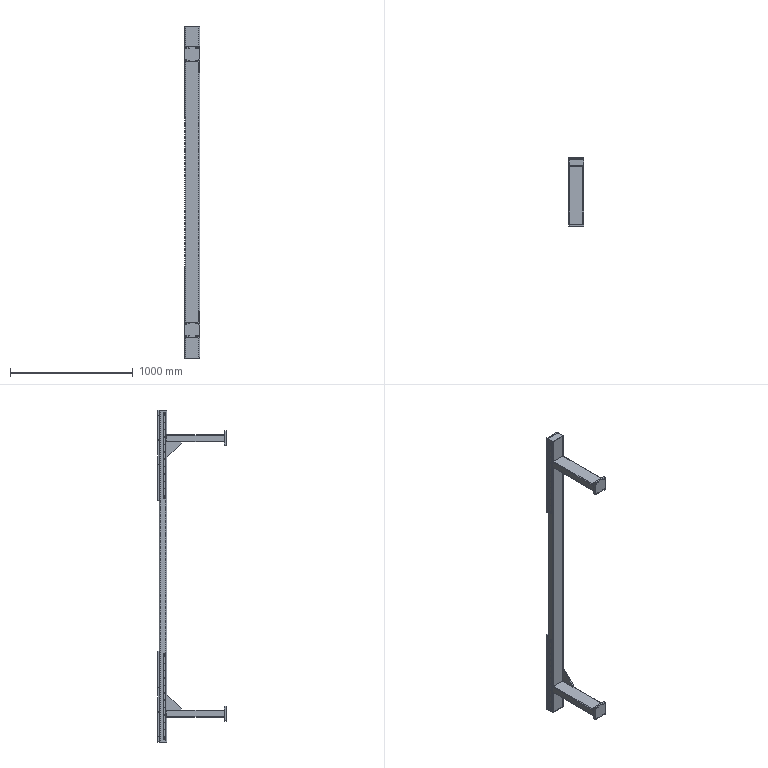Part | SolidWorks | features HoleWzd 6, ICE 6, Chamfer 3, MirrorSolid 3, WeldMemberFeat 2, MirrorPattern 1, WeldCornerFeat 1, WeldmentFeature 1 | 13 solids | 452 faces | box 129.5 x 557 x 2700 mm | volume 6948408 mm3 | cylinder 264 | plane 108 | cone 80 | commonest cylinder face diameters 3.3 x112 5 x64 4.2 x24 6.4 x20 6.8 x16 9 x16